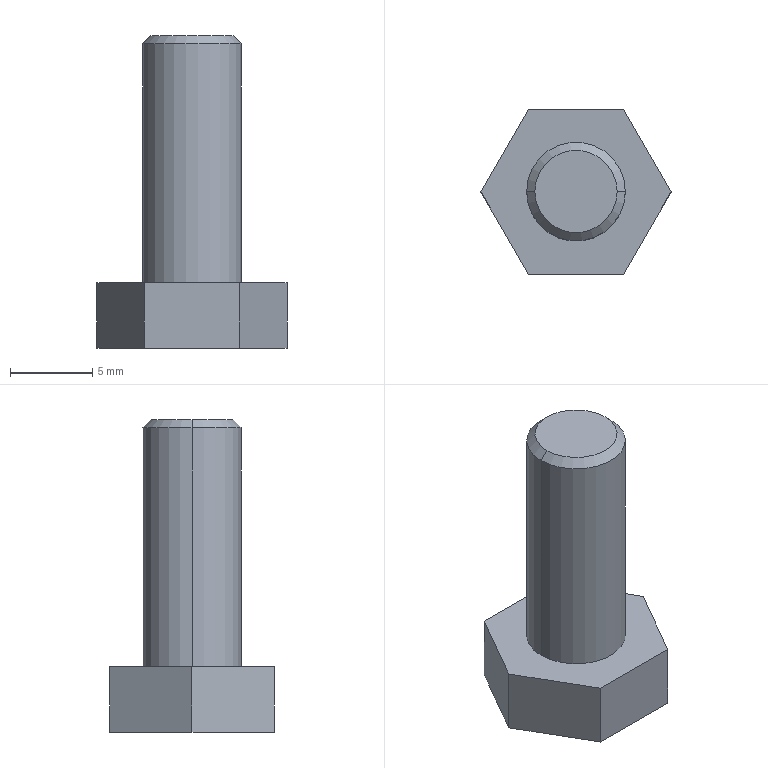Part | STEP file | Bulong M6_1.5F | 1 solid | 13 faces | box 11.547 x 10 x 19 mm | volume 768.3 mm3 | plane 9 | cone 2 | cylinder 2 | commonest cylinder face diameters 6 x2
STEP:
#1=CARTESIAN_POINT('',(0.,0.,0.));
#2=DIRECTION('',(0.,0.,1.));
#3=DIRECTION('',(1.,0.,0.));
#4=AXIS2_PLACEMENT_3D('',#1,#2,#3);
#5=CARTESIAN_POINT('',(2.5,0.,15.));
#6=VERTEX_POINT('',#5);
#7=CARTESIAN_POINT('',(-2.5,0.,15.));
#8=VERTEX_POINT('',#7);
#9=CARTESIAN_POINT('',(0.,0.,15.));
#10=DIRECTION('',(0.,0.,1.));
#11=DIRECTION('',(1.,0.,0.));
#12=AXIS2_PLACEMENT_3D('',#9,#10,#11);
#13=CIRCLE('',#12,2.5);
#14=CARTESIAN_POINT('',(0.,0.,15.));
#15=DIRECTION('',(0.,0.,-1.));
#16=DIRECTION('',(-1.,0.,0.));
#17=AXIS2_PLACEMENT_3D('',#14,#15,#16);
#18=CONICAL_SURFACE('',#17,2.5,0.7854);
#19=CARTESIAN_POINT('',(3.142,0.));
#20=DIRECTION('',(-1.,0.));
#21=VECTOR('',#20,1.);
#22=LINE('',#19,#21);
#23=(GEOMETRIC_REPRESENTATION_CONTEXT(2)PARAMETRIC_REPRESENTATION_CONTEXT()REPRESENTATION_CONTEXT('',''));
#24=DEFINITIONAL_REPRESENTATION('',(#22),#23);
#25=PCURVE('',#18,#24);
#26=CARTESIAN_POINT('',(0.,0.,15.));
#27=DIRECTION('',(0.,0.,1.));
#28=DIRECTION('',(1.,0.,0.));
#29=AXIS2_PLACEMENT_3D('',#26,#27,#28);
#30=PLANE('',#29);
#31=CARTESIAN_POINT('',(0.,0.));
#32=DIRECTION('',(1.,0.));
#33=AXIS2_PLACEMENT_2D('',#31,#32);
#34=CIRCLE('',#33,2.5);
#35=(GEOMETRIC_REPRESENTATION_CONTEXT(2)PARAMETRIC_REPRESENTATION_CONTEXT()REPRESENTATION_CONTEXT('',''));
#36=DEFINITIONAL_REPRESENTATION('',(#34),#35);
#37=PCURVE('',#30,#36);
#38=SURFACE_CURVE('',#13,(#25,#37),.PCURVE_S1.);
#39=EDGE_CURVE('',#6,#8,#38,.T.);
#40=ORIENTED_EDGE('',*,*,#39,.F.);
#41=CARTESIAN_POINT('',(3.,0.,14.5));
#42=VERTEX_POINT('',#41);
#43=CARTESIAN_POINT('',(2.5,0.,15.));
#44=DIRECTION('',(0.7071,0.,-0.7071));
#45=VECTOR('',#44,1.);
#46=LINE('',#43,#45);
#47=CARTESIAN_POINT('',(3.142,0.));
#48=DIRECTION('',(0.,1.));
#49=VECTOR('',#48,1.);
#50=LINE('',#47,#49);
#51=(GEOMETRIC_REPRESENTATION_CONTEXT(2)PARAMETRIC_REPRESENTATION_CONTEXT()REPRESENTATION_CONTEXT('',''));
#52=DEFINITIONAL_REPRESENTATION('',(#50),#51);
#53=PCURVE('',#18,#52);
#54=CARTESIAN_POINT('',(0.,0.,15.));
#55=DIRECTION('',(0.,0.,-1.));
#56=DIRECTION('',(-1.,0.,0.));
#57=AXIS2_PLACEMENT_3D('',#54,#55,#56);
#58=CONICAL_SURFACE('',#57,2.5,0.7854);
#59=CARTESIAN_POINT('',(3.142,0.));
#60=DIRECTION('',(0.,1.));
#61=VECTOR('',#60,1.);
#62=LINE('',#59,#61);
#63=(GEOMETRIC_REPRESENTATION_CONTEXT(2)PARAMETRIC_REPRESENTATION_CONTEXT()REPRESENTATION_CONTEXT('',''));
#64=DEFINITIONAL_REPRESENTATION('',(#62),#63);
#65=PCURVE('',#58,#64);
#66=SURFACE_CURVE('',#46,(#53,#65),.PCURVE_S1.);
#67=EDGE_CURVE('',#6,#42,#66,.T.);
#68=ORIENTED_EDGE('',*,*,#67,.T.);
#69=CARTESIAN_POINT('',(-3.,0.,14.5));
#70=VERTEX_POINT('',#69);
#71=CARTESIAN_POINT('',(0.,0.,14.5));
#72=DIRECTION('',(0.,0.,-1.));
#73=DIRECTION('',(1.,0.,0.));
#74=AXIS2_PLACEMENT_3D('',#71,#72,#73);
#75=CIRCLE('',#74,3.);
#76=CARTESIAN_POINT('',(-3.142,0.5));
#77=DIRECTION('',(1.,0.));
#78=VECTOR('',#77,1.);
#79=LINE('',#76,#78);
#80=(GEOMETRIC_REPRESENTATION_CONTEXT(2)PARAMETRIC_REPRESENTATION_CONTEXT()REPRESENTATION_CONTEXT('',''));
#81=DEFINITIONAL_REPRESENTATION('',(#79),#80);
#82=PCURVE('',#18,#81);
#83=CARTESIAN_POINT('',(0.,0.,15.));
#84=DIRECTION('',(0.,0.,-1.));
#85=DIRECTION('',(-1.,0.,0.));
#86=AXIS2_PLACEMENT_3D('',#83,#84,#85);
#87=CYLINDRICAL_SURFACE('',#86,3.);
#88=CARTESIAN_POINT('',(-3.142,0.5));
#89=DIRECTION('',(1.,0.));
#90=VECTOR('',#89,1.);
#91=LINE('',#88,#90);
#92=(GEOMETRIC_REPRESENTATION_CONTEXT(2)PARAMETRIC_REPRESENTATION_CONTEXT()REPRESENTATION_CONTEXT('',''));
#93=DEFINITIONAL_REPRESENTATION('',(#91),#92);
#94=PCURVE('',#87,#93);
#95=SURFACE_CURVE('',#75,(#82,#94),.PCURVE_S1.);
#96=EDGE_CURVE('',#70,#42,#95,.T.);
#97=ORIENTED_EDGE('',*,*,#96,.F.);
#98=CARTESIAN_POINT('',(-2.5,0.,15.));
#99=DIRECTION('',(-0.7071,0.,-0.7071));
#100=VECTOR('',#99,1.);
#101=LINE('',#98,#100);
#102=CARTESIAN_POINT('',(0.,0.));
#103=DIRECTION('',(0.,1.));
#104=VECTOR('',#103,1.);
#105=LINE('',#102,#104);
#106=(GEOMETRIC_REPRESENTATION_CONTEXT(2)PARAMETRIC_REPRESENTATION_CONTEXT()REPRESENTATION_CONTEXT('',''));
#107=DEFINITIONAL_REPRESENTATION('',(#105),#106);
#108=PCURVE('',#18,#107);
#109=CARTESIAN_POINT('',(6.283,0.));
#110=DIRECTION('',(0.,1.));
#111=VECTOR('',#110,1.);
#112=LINE('',#109,#111);
#113=(GEOMETRIC_REPRESENTATION_CONTEXT(2)PARAMETRIC_REPRESENTATION_CONTEXT()REPRESENTATION_CONTEXT('',''));
#114=DEFINITIONAL_REPRESENTATION('',(#112),#113);
#115=PCURVE('',#58,#114);
#116=SURFACE_CURVE('',#101,(#108,#115),.PCURVE_S1.);
#117=EDGE_CURVE('',#8,#70,#116,.T.);
#118=ORIENTED_EDGE('',*,*,#117,.F.);
#119=EDGE_LOOP('',(#40,#68,#97,#118));
#120=FACE_BOUND('',#119,.T.);
#121=ADVANCED_FACE('',(#120),#18,.T.);
#122=ORIENTED_EDGE('',*,*,#96,.T.);
#123=CARTESIAN_POINT('',(3.,0.,0.));
#124=VERTEX_POINT('',#123);
#125=CARTESIAN_POINT('',(3.,0.,15.));
#126=DIRECTION('',(0.,0.,-1.));
#127=VECTOR('',#126,1.);
#128=LINE('',#125,#127);
#129=CARTESIAN_POINT('',(3.142,0.));
#130=DIRECTION('',(0.,1.));
#131=VECTOR('',#130,1.);
#132=LINE('',#129,#131);
#133=(GEOMETRIC_REPRESENTATION_CONTEXT(2)PARAMETRIC_REPRESENTATION_CONTEXT()REPRESENTATION_CONTEXT('',''));
#134=DEFINITIONAL_REPRESENTATION('',(#132),#133);
#135=PCURVE('',#87,#134);
#136=CARTESIAN_POINT('',(0.,0.,15.));
#137=DIRECTION('',(0.,0.,-1.));
#138=DIRECTION('',(-1.,0.,0.));
#139=AXIS2_PLACEMENT_3D('',#136,#137,#138);
#140=CYLINDRICAL_SURFACE('',#139,3.);
#141=CARTESIAN_POINT('',(3.142,0.));
#142=DIRECTION('',(0.,1.));
#143=VECTOR('',#142,1.);
#144=LINE('',#141,#143);
#145=(GEOMETRIC_REPRESENTATION_CONTEXT(2)PARAMETRIC_REPRESENTATION_CONTEXT()REPRESENTATION_CONTEXT('',''));
#146=DEFINITIONAL_REPRESENTATION('',(#144),#145);
#147=PCURVE('',#140,#146);
#148=SURFACE_CURVE('',#128,(#135,#147),.PCURVE_S1.);
#149=EDGE_CURVE('',#42,#124,#148,.T.);
#150=ORIENTED_EDGE('',*,*,#149,.T.);
#151=CARTESIAN_POINT('',(-3.,0.,0.));
#152=VERTEX_POINT('',#151);
#153=CARTESIAN_POINT('',(0.,0.,0.));
#154=DIRECTION('',(0.,0.,1.));
#155=DIRECTION('',(1.,0.,0.));
#156=AXIS2_PLACEMENT_3D('',#153,#154,#155);
#157=CIRCLE('',#156,3.);
#158=CARTESIAN_POINT('',(3.142,15.));
#159=DIRECTION('',(-1.,0.));
#160=VECTOR('',#159,1.);
#161=LINE('',#158,#160);
#162=(GEOMETRIC_REPRESENTATION_CONTEXT(2)PARAMETRIC_REPRESENTATION_CONTEXT()REPRESENTATION_CONTEXT('',''));
#163=DEFINITIONAL_REPRESENTATION('',(#161),#162);
#164=PCURVE('',#87,#163);
#165=CARTESIAN_POINT('',(0.,0.,0.));
#166=DIRECTION('',(0.,0.,1.));
#167=DIRECTION('',(1.,0.,0.));
#168=AXIS2_PLACEMENT_3D('',#165,#166,#167);
#169=PLANE('',#168);
#170=CARTESIAN_POINT('',(0.,0.));
#171=DIRECTION('',(1.,0.));
#172=AXIS2_PLACEMENT_2D('',#170,#171);
#173=CIRCLE('',#172,3.);
#174=(GEOMETRIC_REPRESENTATION_CONTEXT(2)PARAMETRIC_REPRESENTATION_CONTEXT()REPRESENTATION_CONTEXT('',''));
#175=DEFINITIONAL_REPRESENTATION('',(#173),#174);
#176=PCURVE('',#169,#175);
#177=SURFACE_CURVE('',#157,(#164,#176),.PCURVE_S1.);
#178=EDGE_CURVE('',#124,#152,#177,.T.);
#179=ORIENTED_EDGE('',*,*,#178,.T.);
#180=CARTESIAN_POINT('',(-3.,0.,15.));
#181=DIRECTION('',(0.,0.,-1.));
#182=VECTOR('',#181,1.);
#183=LINE('',#180,#182);
#184=CARTESIAN_POINT('',(0.,0.));
#185=DIRECTION('',(0.,1.));
#186=VECTOR('',#185,1.);
#187=LINE('',#184,#186);
#188=(GEOMETRIC_REPRESENTATION_CONTEXT(2)PARAMETRIC_REPRESENTATION_CONTEXT()REPRESENTATION_CONTEXT('',''));
#189=DEFINITIONAL_REPRESENTATION('',(#187),#188);
#190=PCURVE('',#87,#189);
#191=CARTESIAN_POINT('',(6.283,0.));
#192=DIRECTION('',(0.,1.));
#193=VECTOR('',#192,1.);
#194=LINE('',#191,#193);
#195=(GEOMETRIC_REPRESENTATION_CONTEXT(2)PARAMETRIC_REPRESENTATION_CONTEXT()REPRESENTATION_CONTEXT('',''));
#196=DEFINITIONAL_REPRESENTATION('',(#194),#195);
#197=PCURVE('',#140,#196);
#198=SURFACE_CURVE('',#183,(#190,#197),.PCURVE_S1.);
#199=EDGE_CURVE('',#70,#152,#198,.T.);
#200=ORIENTED_EDGE('',*,*,#199,.F.);
#201=EDGE_LOOP('',(#122,#150,#179,#200));
#202=FACE_BOUND('',#201,.T.);
#203=ADVANCED_FACE('',(#202),#87,.T.);
#204=CARTESIAN_POINT('',(-2.887,5.,0.));
#205=VERTEX_POINT('',#204);
#206=CARTESIAN_POINT('',(-5.774,0.,0.));
#207=VERTEX_POINT('',#206);
#208=CARTESIAN_POINT('',(-2.887,5.,0.));
#209=DIRECTION('',(-0.5,-0.866,0.));
#210=VECTOR('',#209,1.);
#211=LINE('',#208,#210);
#212=CARTESIAN_POINT('',(-2.887,5.));
#213=DIRECTION('',(-0.5,-0.866));
#214=VECTOR('',#213,1.);
#215=LINE('',#212,#214);
#216=(GEOMETRIC_REPRESENTATION_CONTEXT(2)PARAMETRIC_REPRESENTATION_CONTEXT()REPRESENTATION_CONTEXT('',''));
#217=DEFINITIONAL_REPRESENTATION('',(#215),#216);
#218=PCURVE('',#169,#217);
#219=CARTESIAN_POINT('',(-2.887,5.,-4.));
#220=DIRECTION('',(-0.866,0.5,0.));
#221=DIRECTION('',(-0.5,-0.866,0.));
#222=AXIS2_PLACEMENT_3D('',#219,#220,#221);
#223=PLANE('',#222);
#224=CARTESIAN_POINT('',(0.,4.));
#225=DIRECTION('',(1.,0.));
#226=VECTOR('',#225,1.);
#227=LINE('',#224,#226);
#228=(GEOMETRIC_REPRESENTATION_CONTEXT(2)PARAMETRIC_REPRESENTATION_CONTEXT()REPRESENTATION_CONTEXT('',''));
#229=DEFINITIONAL_REPRESENTATION('',(#227),#228);
#230=PCURVE('',#223,#229);
#231=SURFACE_CURVE('',#211,(#218,#230),.PCURVE_S1.);
#232=EDGE_CURVE('',#205,#207,#231,.T.);
#233=ORIENTED_EDGE('',*,*,#232,.T.);
#234=CARTESIAN_POINT('',(-2.887,-5.,0.));
#235=VERTEX_POINT('',#234);
#236=CARTESIAN_POINT('',(-5.774,0.,0.));
#237=DIRECTION('',(0.5,-0.866,0.));
#238=VECTOR('',#237,1.);
#239=LINE('',#236,#238);
#240=CARTESIAN_POINT('',(-5.774,0.));
#241=DIRECTION('',(0.5,-0.866));
#242=VECTOR('',#241,1.);
#243=LINE('',#240,#242);
#244=(GEOMETRIC_REPRESENTATION_CONTEXT(2)PARAMETRIC_REPRESENTATION_CONTEXT()REPRESENTATION_CONTEXT('',''));
#245=DEFINITIONAL_REPRESENTATION('',(#243),#244);
#246=PCURVE('',#169,#245);
#247=CARTESIAN_POINT('',(-5.774,0.,-4.));
#248=DIRECTION('',(-0.866,-0.5,0.));
#249=DIRECTION('',(0.5,-0.866,0.));
#250=AXIS2_PLACEMENT_3D('',#247,#248,#249);
#251=PLANE('',#250);
#252=CARTESIAN_POINT('',(0.,4.));
#253=DIRECTION('',(1.,0.));
#254=VECTOR('',#253,1.);
#255=LINE('',#252,#254);
#256=(GEOMETRIC_REPRESENTATION_CONTEXT(2)PARAMETRIC_REPRESENTATION_CONTEXT()REPRESENTATION_CONTEXT('',''));
#257=DEFINITIONAL_REPRESENTATION('',(#255),#256);
#258=PCURVE('',#251,#257);
#259=SURFACE_CURVE('',#239,(#246,#258),.PCURVE_S1.);
#260=EDGE_CURVE('',#207,#235,#259,.T.);
#261=ORIENTED_EDGE('',*,*,#260,.T.);
#262=CARTESIAN_POINT('',(2.887,-5.,0.));
#263=VERTEX_POINT('',#262);
#264=CARTESIAN_POINT('',(-2.887,-5.,0.));
#265=DIRECTION('',(1.,0.,0.));
#266=VECTOR('',#265,1.);
#267=LINE('',#264,#266);
#268=CARTESIAN_POINT('',(-2.887,-5.));
#269=DIRECTION('',(1.,0.));
#270=VECTOR('',#269,1.);
#271=LINE('',#268,#270);
#272=(GEOMETRIC_REPRESENTATION_CONTEXT(2)PARAMETRIC_REPRESENTATION_CONTEXT()REPRESENTATION_CONTEXT('',''));
#273=DEFINITIONAL_REPRESENTATION('',(#271),#272);
#274=PCURVE('',#169,#273);
#275=CARTESIAN_POINT('',(-2.887,-5.,-4.));
#276=DIRECTION('',(0.,-1.,0.));
#277=DIRECTION('',(1.,0.,0.));
#278=AXIS2_PLACEMENT_3D('',#275,#276,#277);
#279=PLANE('',#278);
#280=CARTESIAN_POINT('',(0.,4.));
#281=DIRECTION('',(1.,0.));
#282=VECTOR('',#281,1.);
#283=LINE('',#280,#282);
#284=(GEOMETRIC_REPRESENTATION_CONTEXT(2)PARAMETRIC_REPRESENTATION_CONTEXT()REPRESENTATION_CONTEXT('',''));
#285=DEFINITIONAL_REPRESENTATION('',(#283),#284);
#286=PCURVE('',#279,#285);
#287=SURFACE_CURVE('',#267,(#274,#286),.PCURVE_S1.);
#288=EDGE_CURVE('',#235,#263,#287,.T.);
#289=ORIENTED_EDGE('',*,*,#288,.T.);
#290=CARTESIAN_POINT('',(5.774,0.,0.));
#291=VERTEX_POINT('',#290);
#292=CARTESIAN_POINT('',(2.887,-5.,0.));
#293=DIRECTION('',(0.5,0.866,0.));
#294=VECTOR('',#293,1.);
#295=LINE('',#292,#294);
#296=CARTESIAN_POINT('',(2.887,-5.));
#297=DIRECTION('',(0.5,0.866));
#298=VECTOR('',#297,1.);
#299=LINE('',#296,#298);
#300=(GEOMETRIC_REPRESENTATION_CONTEXT(2)PARAMETRIC_REPRESENTATION_CONTEXT()REPRESENTATION_CONTEXT('',''));
#301=DEFINITIONAL_REPRESENTATION('',(#299),#300);
#302=PCURVE('',#169,#301);
#303=CARTESIAN_POINT('',(2.887,-5.,-4.));
#304=DIRECTION('',(0.866,-0.5,0.));
#305=DIRECTION('',(0.5,0.866,0.));
#306=AXIS2_PLACEMENT_3D('',#303,#304,#305);
#307=PLANE('',#306);
#308=CARTESIAN_POINT('',(0.,4.));
#309=DIRECTION('',(1.,0.));
#310=VECTOR('',#309,1.);
#311=LINE('',#308,#310);
#312=(GEOMETRIC_REPRESENTATION_CONTEXT(2)PARAMETRIC_REPRESENTATION_CONTEXT()REPRESENTATION_CONTEXT('',''));
#313=DEFINITIONAL_REPRESENTATION('',(#311),#312);
#314=PCURVE('',#307,#313);
#315=SURFACE_CURVE('',#295,(#302,#314),.PCURVE_S1.);
#316=EDGE_CURVE('',#263,#291,#315,.T.);
#317=ORIENTED_EDGE('',*,*,#316,.T.);
#318=CARTESIAN_POINT('',(2.887,5.,0.));
#319=VERTEX_POINT('',#318);
#320=CARTESIAN_POINT('',(5.774,0.,0.));
#321=DIRECTION('',(-0.5,0.866,0.));
#322=VECTOR('',#321,1.);
#323=LINE('',#320,#322);
#324=CARTESIAN_POINT('',(5.774,0.));
#325=DIRECTION('',(-0.5,0.866));
#326=VECTOR('',#325,1.);
#327=LINE('',#324,#326);
#328=(GEOMETRIC_REPRESENTATION_CONTEXT(2)PARAMETRIC_REPRESENTATION_CONTEXT()REPRESENTATION_CONTEXT('',''));
#329=DEFINITIONAL_REPRESENTATION('',(#327),#328);
#330=PCURVE('',#169,#329);
#331=CARTESIAN_POINT('',(5.774,0.,-4.));
#332=DIRECTION('',(0.866,0.5,0.));
#333=DIRECTION('',(-0.5,0.866,0.));
#334=AXIS2_PLACEMENT_3D('',#331,#332,#333);
#335=PLANE('',#334);
#336=CARTESIAN_POINT('',(0.,4.));
#337=DIRECTION('',(1.,0.));
#338=VECTOR('',#337,1.);
#339=LINE('',#336,#338);
#340=(GEOMETRIC_REPRESENTATION_CONTEXT(2)PARAMETRIC_REPRESENTATION_CONTEXT()REPRESENTATION_CONTEXT('',''));
#341=DEFINITIONAL_REPRESENTATION('',(#339),#340);
#342=PCURVE('',#335,#341);
#343=SURFACE_CURVE('',#323,(#330,#342),.PCURVE_S1.);
#344=EDGE_CURVE('',#291,#319,#343,.T.);
#345=ORIENTED_EDGE('',*,*,#344,.T.);
#346=CARTESIAN_POINT('',(2.887,5.,0.));
#347=DIRECTION('',(-1.,0.,0.));
#348=VECTOR('',#347,1.);
#349=LINE('',#346,#348);
#350=CARTESIAN_POINT('',(2.887,5.));
#351=DIRECTION('',(-1.,0.));
#352=VECTOR('',#351,1.);
#353=LINE('',#350,#352);
#354=(GEOMETRIC_REPRESENTATION_CONTEXT(2)PARAMETRIC_REPRESENTATION_CONTEXT()REPRESENTATION_CONTEXT('',''));
#355=DEFINITIONAL_REPRESENTATION('',(#353),#354);
#356=PCURVE('',#169,#355);
#357=CARTESIAN_POINT('',(2.887,5.,-4.));
#358=DIRECTION('',(0.,1.,0.));
#359=DIRECTION('',(0.,0.,1.));
#360=AXIS2_PLACEMENT_3D('',#357,#358,#359);
#361=PLANE('',#360);
#362=CARTESIAN_POINT('',(4.,0.));
#363=DIRECTION('',(0.,-1.));
#364=VECTOR('',#363,1.);
#365=LINE('',#362,#364);
#366=(GEOMETRIC_REPRESENTATION_CONTEXT(2)PARAMETRIC_REPRESENTATION_CONTEXT()REPRESENTATION_CONTEXT('',''));
#367=DEFINITIONAL_REPRESENTATION('',(#365),#366);
#368=PCURVE('',#361,#367);
#369=SURFACE_CURVE('',#349,(#356,#368),.PCURVE_S1.);
#370=EDGE_CURVE('',#319,#205,#369,.T.);
#371=ORIENTED_EDGE('',*,*,#370,.T.);
#372=EDGE_LOOP('',(#233,#261,#289,#317,#345,#371));
#373=FACE_BOUND('',#372,.T.);
#374=CARTESIAN_POINT('',(0.,0.,0.));
#375=DIRECTION('',(0.,0.,1.));
#376=DIRECTION('',(1.,0.,0.));
#377=AXIS2_PLACEMENT_3D('',#374,#375,#376);
#378=CIRCLE('',#377,3.);
#379=CARTESIAN_POINT('',(0.,0.));
#380=DIRECTION('',(1.,0.));
#381=AXIS2_PLACEMENT_2D('',#379,#380);
#382=CIRCLE('',#381,3.);
#383=(GEOMETRIC_REPRESENTATION_CONTEXT(2)PARAMETRIC_REPRESENTATION_CONTEXT()REPRESENTATION_CONTEXT('',''));
#384=DEFINITIONAL_REPRESENTATION('',(#382),#383);
#385=PCURVE('',#169,#384);
#386=CARTESIAN_POINT('',(9.425,15.));
#387=DIRECTION('',(-1.,0.));
#388=VECTOR('',#387,1.);
#389=LINE('',#386,#388);
#390=(GEOMETRIC_REPRESENTATION_CONTEXT(2)PARAMETRIC_REPRESENTATION_CONTEXT()REPRESENTATION_CONTEXT('',''));
#391=DEFINITIONAL_REPRESENTATION('',(#389),#390);
#392=PCURVE('',#140,#391);
#393=SURFACE_CURVE('',#378,(#385,#392),.PCURVE_S1.);
#394=EDGE_CURVE('',#152,#124,#393,.T.);
#395=ORIENTED_EDGE('',*,*,#394,.F.);
#396=ORIENTED_EDGE('',*,*,#178,.F.);
#397=EDGE_LOOP('',(#395,#396));
#398=FACE_BOUND('',#397,.T.);
#399=ADVANCED_FACE('',(#373,#398),#169,.T.);
#400=ORIENTED_EDGE('',*,*,#232,.F.);
#401=CARTESIAN_POINT('',(-2.887,5.,-4.));
#402=VERTEX_POINT('',#401);
#403=CARTESIAN_POINT('',(-2.887,5.,-4.));
#404=DIRECTION('',(0.,0.,1.));
#405=VECTOR('',#404,1.);
#406=LINE('',#403,#405);
#407=CARTESIAN_POINT('',(0.,0.));
#408=DIRECTION('',(0.,1.));
#409=VECTOR('',#408,1.);
#410=LINE('',#407,#409);
#411=(GEOMETRIC_REPRESENTATION_CONTEXT(2)PARAMETRIC_REPRESENTATION_CONTEXT()REPRESENTATION_CONTEXT('',''));
#412=DEFINITIONAL_REPRESENTATION('',(#410),#411);
#413=PCURVE('',#223,#412);
#414=CARTESIAN_POINT('',(0.,-5.774));
#415=DIRECTION('',(1.,0.));
#416=VECTOR('',#415,1.);
#417=LINE('',#414,#416);
#418=(GEOMETRIC_REPRESENTATION_CONTEXT(2)PARAMETRIC_REPRESENTATION_CONTEXT()REPRESENTATION_CONTEXT('',''));
#419=DEFINITIONAL_REPRESENTATION('',(#417),#418);
#420=PCURVE('',#361,#419);
#421=SURFACE_CURVE('',#406,(#413,#420),.PCURVE_S1.);
#422=EDGE_CURVE('',#402,#205,#421,.T.);
#423=ORIENTED_EDGE('',*,*,#422,.F.);
#424=CARTESIAN_POINT('',(-5.774,0.,-4.));
#425=VERTEX_POINT('',#424);
#426=CARTESIAN_POINT('',(-2.887,5.,-4.));
#427=DIRECTION('',(-0.5,-0.866,0.));
#428=VECTOR('',#427,1.);
#429=LINE('',#426,#428);
#430=CARTESIAN_POINT('',(0.,0.));
#431=DIRECTION('',(1.,0.));
#432=VECTOR('',#431,1.);
#433=LINE('',#430,#432);
#434=(GEOMETRIC_REPRESENTATION_CONTEXT(2)PARAMETRIC_REPRESENTATION_CONTEXT()REPRESENTATION_CONTEXT('',''));
#435=DEFINITIONAL_REPRESENTATION('',(#433),#434);
#436=PCURVE('',#223,#435);
#437=CARTESIAN_POINT('',(0.,0.,-4.));
#438=DIRECTION('',(0.,0.,1.));
#439=DIRECTION('',(1.,0.,0.));
#440=AXIS2_PLACEMENT_3D('',#437,#438,#439);
#441=PLANE('',#440);
#442=CARTESIAN_POINT('',(-2.887,5.));
#443=DIRECTION('',(-0.5,-0.866));
#444=VECTOR('',#443,1.);
#445=LINE('',#442,#444);
#446=(GEOMETRIC_REPRESENTATION_CONTEXT(2)PARAMETRIC_REPRESENTATION_CONTEXT()REPRESENTATION_CONTEXT('',''));
#447=DEFINITIONAL_REPRESENTATION('',(#445),#446);
#448=PCURVE('',#441,#447);
#449=SURFACE_CURVE('',#429,(#436,#448),.PCURVE_S1.);
#450=EDGE_CURVE('',#402,#425,#449,.T.);
#451=ORIENTED_EDGE('',*,*,#450,.T.);
#452=CARTESIAN_POINT('',(-5.774,0.,-4.));
#453=DIRECTION('',(0.,0.,1.));
#454=VECTOR('',#453,1.);
#455=LINE('',#452,#454);
#456=CARTESIAN_POINT('',(5.774,0.));
#457=DIRECTION('',(0.,1.));
#458=VECTOR('',#457,1.);
#459=LINE('',#456,#458);
#460=(GEOMETRIC_REPRESENTATION_CONTEXT(2)PARAMETRIC_REPRESENTATION_CONTEXT()REPRESENTATION_CONTEXT('',''));
#461=DEFINITIONAL_REPRESENTATION('',(#459),#460);
#462=PCURVE('',#223,#461);
#463=CARTESIAN_POINT('',(0.,0.));
#464=DIRECTION('',(0.,1.));
#465=VECTOR('',#464,1.);
#466=LINE('',#463,#465);
#467=(GEOMETRIC_REPRESENTATION_CONTEXT(2)PARAMETRIC_REPRESENTATION_CONTEXT()REPRESENTATION_CONTEXT('',''));
#468=DEFINITIONAL_REPRESENTATION('',(#466),#467);
#469=PCURVE('',#251,#468);
#470=SURFACE_CURVE('',#455,(#462,#469),.PCURVE_S1.);
#471=EDGE_CURVE('',#425,#207,#470,.T.);
#472=ORIENTED_EDGE('',*,*,#471,.T.);
#473=EDGE_LOOP('',(#400,#423,#451,#472));
#474=FACE_BOUND('',#473,.T.);
#475=ADVANCED_FACE('',(#474),#223,.T.);
#476=ORIENTED_EDGE('',*,*,#370,.F.);
#477=CARTESIAN_POINT('',(2.887,5.,-4.));
#478=VERTEX_POINT('',#477);
#479=CARTESIAN_POINT('',(2.887,5.,-4.));
#480=DIRECTION('',(0.,0.,1.));
#481=VECTOR('',#480,1.);
#482=LINE('',#479,#481);
#483=CARTESIAN_POINT('',(0.,0.));
#484=DIRECTION('',(1.,0.));
#485=VECTOR('',#484,1.);
#486=LINE('',#483,#485);
#487=(GEOMETRIC_REPRESENTATION_CONTEXT(2)PARAMETRIC_REPRESENTATION_CONTEXT()REPRESENTATION_CONTEXT('',''));
#488=DEFINITIONAL_REPRESENTATION('',(#486),#487);
#489=PCURVE('',#361,#488);
#490=CARTESIAN_POINT('',(5.774,0.));
#491=DIRECTION('',(0.,1.));
#492=VECTOR('',#491,1.);
#493=LINE('',#490,#492);
#494=(GEOMETRIC_REPRESENTATION_CONTEXT(2)PARAMETRIC_REPRESENTATION_CONTEXT()REPRESENTATION_CONTEXT('',''));
#495=DEFINITIONAL_REPRESENTATION('',(#493),#494);
#496=PCURVE('',#335,#495);
#497=SURFACE_CURVE('',#482,(#489,#496),.PCURVE_S1.);
#498=EDGE_CURVE('',#478,#319,#497,.T.);
#499=ORIENTED_EDGE('',*,*,#498,.F.);
#500=CARTESIAN_POINT('',(2.887,5.,-4.));
#501=DIRECTION('',(-1.,0.,0.));
#502=VECTOR('',#501,1.);
#503=LINE('',#500,#502);
#504=CARTESIAN_POINT('',(0.,0.));
#505=DIRECTION('',(0.,-1.));
#506=VECTOR('',#505,1.);
#507=LINE('',#504,#506);
#508=(GEOMETRIC_REPRESENTATION_CONTEXT(2)PARAMETRIC_REPRESENTATION_CONTEXT()REPRESENTATION_CONTEXT('',''));
#509=DEFINITIONAL_REPRESENTATION('',(#507),#508);
#510=PCURVE('',#361,#509);
#511=CARTESIAN_POINT('',(2.887,5.));
#512=DIRECTION('',(-1.,0.));
#513=VECTOR('',#512,1.);
#514=LINE('',#511,#513);
#515=(GEOMETRIC_REPRESENTATION_CONTEXT(2)PARAMETRIC_REPRESENTATION_CONTEXT()REPRESENTATION_CONTEXT('',''));
#516=DEFINITIONAL_REPRESENTATION('',(#514),#515);
#517=PCURVE('',#441,#516);
#518=SURFACE_CURVE('',#503,(#510,#517),.PCURVE_S1.);
#519=EDGE_CURVE('',#478,#402,#518,.T.);
#520=ORIENTED_EDGE('',*,*,#519,.T.);
#521=ORIENTED_EDGE('',*,*,#422,.T.);
#522=EDGE_LOOP('',(#476,#499,#520,#521));
#523=FACE_BOUND('',#522,.T.);
#524=ADVANCED_FACE('',(#523),#361,.T.);
#525=ORIENTED_EDGE('',*,*,#344,.F.);
#526=CARTESIAN_POINT('',(5.774,0.,-4.));
#527=VERTEX_POINT('',#526);
#528=CARTESIAN_POINT('',(5.774,0.,-4.));
#529=DIRECTION('',(0.,0.,1.));
#530=VECTOR('',#529,1.);
#531=LINE('',#528,#530);
#532=CARTESIAN_POINT('',(0.,0.));
#533=DIRECTION('',(0.,1.));
#534=VECTOR('',#533,1.);
#535=LINE('',#532,#534);
#536=(GEOMETRIC_REPRESENTATION_CONTEXT(2)PARAMETRIC_REPRESENTATION_CONTEXT()REPRESENTATION_CONTEXT('',''));
#537=DEFINITIONAL_REPRESENTATION('',(#535),#536);
#538=PCURVE('',#335,#537);
#539=CARTESIAN_POINT('',(5.774,0.));
#540=DIRECTION('',(0.,1.));
#541=VECTOR('',#540,1.);
#542=LINE('',#539,#541);
#543=(GEOMETRIC_REPRESENTATION_CONTEXT(2)PARAMETRIC_REPRESENTATION_CONTEXT()REPRESENTATION_CONTEXT('',''));
#544=DEFINITIONAL_REPRESENTATION('',(#542),#543);
#545=PCURVE('',#307,#544);
#546=SURFACE_CURVE('',#531,(#538,#545),.PCURVE_S1.);
#547=EDGE_CURVE('',#527,#291,#546,.T.);
#548=ORIENTED_EDGE('',*,*,#547,.F.);
#549=CARTESIAN_POINT('',(5.774,0.,-4.));
#550=DIRECTION('',(-0.5,0.866,0.));
#551=VECTOR('',#550,1.);
#552=LINE('',#549,#551);
#553=CARTESIAN_POINT('',(0.,0.));
#554=DIRECTION('',(1.,0.));
#555=VECTOR('',#554,1.);
#556=LINE('',#553,#555);
#557=(GEOMETRIC_REPRESENTATION_CONTEXT(2)PARAMETRIC_REPRESENTATION_CONTEXT()REPRESENTATION_CONTEXT('',''));
#558=DEFINITIONAL_REPRESENTATION('',(#556),#557);
#559=PCURVE('',#335,#558);
#560=CARTESIAN_POINT('',(5.774,0.));
#561=DIRECTION('',(-0.5,0.866));
#562=VECTOR('',#561,1.);
#563=LINE('',#560,#562);
#564=(GEOMETRIC_REPRESENTATION_CONTEXT(2)PARAMETRIC_REPRESENTATION_CONTEXT()REPRESENTATION_CONTEXT('',''));
#565=DEFINITIONAL_REPRESENTATION('',(#563),#564);
#566=PCURVE('',#441,#565);
#567=SURFACE_CURVE('',#552,(#559,#566),.PCURVE_S1.);
#568=EDGE_CURVE('',#527,#478,#567,.T.);
#569=ORIENTED_EDGE('',*,*,#568,.T.);
#570=ORIENTED_EDGE('',*,*,#498,.T.);
#571=EDGE_LOOP('',(#525,#548,#569,#570));
#572=FACE_BOUND('',#571,.T.);
#573=ADVANCED_FACE('',(#572),#335,.T.);
#574=ORIENTED_EDGE('',*,*,#316,.F.);
#575=CARTESIAN_POINT('',(2.887,-5.,-4.));
#576=VERTEX_POINT('',#575);
#577=CARTESIAN_POINT('',(2.887,-5.,-4.));
#578=DIRECTION('',(0.,0.,1.));
#579=VECTOR('',#578,1.);
#580=LINE('',#577,#579);
#581=CARTESIAN_POINT('',(0.,0.));
#582=DIRECTION('',(0.,1.));
#583=VECTOR('',#582,1.);
#584=LINE('',#581,#583);
#585=(GEOMETRIC_REPRESENTATION_CONTEXT(2)PARAMETRIC_REPRESENTATION_CONTEXT()REPRESENTATION_CONTEXT('',''));
#586=DEFINITIONAL_REPRESENTATION('',(#584),#585);
#587=PCURVE('',#307,#586);
#588=CARTESIAN_POINT('',(5.774,0.));
#589=DIRECTION('',(0.,1.));
#590=VECTOR('',#589,1.);
#591=LINE('',#588,#590);
#592=(GEOMETRIC_REPRESENTATION_CONTEXT(2)PARAMETRIC_REPRESENTATION_CONTEXT()REPRESENTATION_CONTEXT('',''));
#593=DEFINITIONAL_REPRESENTATION('',(#591),#592);
#594=PCURVE('',#279,#593);
#595=SURFACE_CURVE('',#580,(#587,#594),.PCURVE_S1.);
#596=EDGE_CURVE('',#576,#263,#595,.T.);
#597=ORIENTED_EDGE('',*,*,#596,.F.);
#598=CARTESIAN_POINT('',(2.887,-5.,-4.));
#599=DIRECTION('',(0.5,0.866,0.));
#600=VECTOR('',#599,1.);
#601=LINE('',#598,#600);
#602=CARTESIAN_POINT('',(0.,0.));
#603=DIRECTION('',(1.,0.));
#604=VECTOR('',#603,1.);
#605=LINE('',#602,#604);
#606=(GEOMETRIC_REPRESENTATION_CONTEXT(2)PARAMETRIC_REPRESENTATION_CONTEXT()REPRESENTATION_CONTEXT('',''));
#607=DEFINITIONAL_REPRESENTATION('',(#605),#606);
#608=PCURVE('',#307,#607);
#609=CARTESIAN_POINT('',(2.887,-5.));
#610=DIRECTION('',(0.5,0.866));
#611=VECTOR('',#610,1.);
#612=LINE('',#609,#611);
#613=(GEOMETRIC_REPRESENTATION_CONTEXT(2)PARAMETRIC_REPRESENTATION_CONTEXT()REPRESENTATION_CONTEXT('',''));
#614=DEFINITIONAL_REPRESENTATION('',(#612),#613);
#615=PCURVE('',#441,#614);
#616=SURFACE_CURVE('',#601,(#608,#615),.PCURVE_S1.);
#617=EDGE_CURVE('',#576,#527,#616,.T.);
#618=ORIENTED_EDGE('',*,*,#617,.T.);
#619=ORIENTED_EDGE('',*,*,#547,.T.);
#620=EDGE_LOOP('',(#574,#597,#618,#619));
#621=FACE_BOUND('',#620,.T.);
#622=ADVANCED_FACE('',(#621),#307,.T.);
#623=ORIENTED_EDGE('',*,*,#288,.F.);
#624=CARTESIAN_POINT('',(-2.887,-5.,-4.));
#625=VERTEX_POINT('',#624);
#626=CARTESIAN_POINT('',(-2.887,-5.,-4.));
#627=DIRECTION('',(0.,0.,1.));
#628=VECTOR('',#627,1.);
#629=LINE('',#626,#628);
#630=CARTESIAN_POINT('',(0.,0.));
#631=DIRECTION('',(0.,1.));
#632=VECTOR('',#631,1.);
#633=LINE('',#630,#632);
#634=(GEOMETRIC_REPRESENTATION_CONTEXT(2)PARAMETRIC_REPRESENTATION_CONTEXT()REPRESENTATION_CONTEXT('',''));
#635=DEFINITIONAL_REPRESENTATION('',(#633),#634);
#636=PCURVE('',#279,#635);
#637=CARTESIAN_POINT('',(5.774,0.));
#638=DIRECTION('',(0.,1.));
#639=VECTOR('',#638,1.);
#640=LINE('',#637,#639);
#641=(GEOMETRIC_REPRESENTATION_CONTEXT(2)PARAMETRIC_REPRESENTATION_CONTEXT()REPRESENTATION_CONTEXT('',''));
#642=DEFINITIONAL_REPRESENTATION('',(#640),#641);
#643=PCURVE('',#251,#642);
#644=SURFACE_CURVE('',#629,(#636,#643),.PCURVE_S1.);
#645=EDGE_CURVE('',#625,#235,#644,.T.);
#646=ORIENTED_EDGE('',*,*,#645,.F.);
#647=CARTESIAN_POINT('',(-2.887,-5.,-4.));
#648=DIRECTION('',(1.,0.,0.));
#649=VECTOR('',#648,1.);
#650=LINE('',#647,#649);
#651=CARTESIAN_POINT('',(0.,0.));
#652=DIRECTION('',(1.,0.));
#653=VECTOR('',#652,1.);
#654=LINE('',#651,#653);
#655=(GEOMETRIC_REPRESENTATION_CONTEXT(2)PARAMETRIC_REPRESENTATION_CONTEXT()REPRESENTATION_CONTEXT('',''));
#656=DEFINITIONAL_REPRESENTATION('',(#654),#655);
#657=PCURVE('',#279,#656);
#658=CARTESIAN_POINT('',(-2.887,-5.));
#659=DIRECTION('',(1.,0.));
#660=VECTOR('',#659,1.);
#661=LINE('',#658,#660);
#662=(GEOMETRIC_REPRESENTATION_CONTEXT(2)PARAMETRIC_REPRESENTATION_CONTEXT()REPRESENTATION_CONTEXT('',''));
#663=DEFINITIONAL_REPRESENTATION('',(#661),#662);
#664=PCURVE('',#441,#663);
#665=SURFACE_CURVE('',#650,(#657,#664),.PCURVE_S1.);
#666=EDGE_CURVE('',#625,#576,#665,.T.);
#667=ORIENTED_EDGE('',*,*,#666,.T.);
#668=ORIENTED_EDGE('',*,*,#596,.T.);
#669=EDGE_LOOP('',(#623,#646,#667,#668));
#670=FACE_BOUND('',#669,.T.);
#671=ADVANCED_FACE('',(#670),#279,.T.);
#672=ORIENTED_EDGE('',*,*,#260,.F.);
#673=ORIENTED_EDGE('',*,*,#471,.F.);
#674=CARTESIAN_POINT('',(-5.774,0.,-4.));
#675=DIRECTION('',(0.5,-0.866,0.));
#676=VECTOR('',#675,1.);
#677=LINE('',#674,#676);
#678=CARTESIAN_POINT('',(0.,0.));
#679=DIRECTION('',(1.,0.));
#680=VECTOR('',#679,1.);
#681=LINE('',#678,#680);
#682=(GEOMETRIC_REPRESENTATION_CONTEXT(2)PARAMETRIC_REPRESENTATION_CONTEXT()REPRESENTATION_CONTEXT('',''));
#683=DEFINITIONAL_REPRESENTATION('',(#681),#682);
#684=PCURVE('',#251,#683);
#685=CARTESIAN_POINT('',(-5.774,0.));
#686=DIRECTION('',(0.5,-0.866));
#687=VECTOR('',#686,1.);
#688=LINE('',#685,#687);
#689=(GEOMETRIC_REPRESENTATION_CONTEXT(2)PARAMETRIC_REPRESENTATION_CONTEXT()REPRESENTATION_CONTEXT('',''));
#690=DEFINITIONAL_REPRESENTATION('',(#688),#689);
#691=PCURVE('',#441,#690);
#692=SURFACE_CURVE('',#677,(#684,#691),.PCURVE_S1.);
#693=EDGE_CURVE('',#425,#625,#692,.T.);
#694=ORIENTED_EDGE('',*,*,#693,.T.);
#695=ORIENTED_EDGE('',*,*,#645,.T.);
#696=EDGE_LOOP('',(#672,#673,#694,#695));
#697=FACE_BOUND('',#696,.T.);
#698=ADVANCED_FACE('',(#697),#251,.T.);
#699=ORIENTED_EDGE('',*,*,#450,.F.);
#700=ORIENTED_EDGE('',*,*,#519,.F.);
#701=ORIENTED_EDGE('',*,*,#568,.F.);
#702=ORIENTED_EDGE('',*,*,#617,.F.);
#703=ORIENTED_EDGE('',*,*,#666,.F.);
#704=ORIENTED_EDGE('',*,*,#693,.F.);
#705=EDGE_LOOP('',(#699,#700,#701,#702,#703,#704));
#706=FACE_BOUND('',#705,.T.);
#707=ADVANCED_FACE('',(#706),#441,.F.);
#708=ORIENTED_EDGE('',*,*,#149,.F.);
#709=CARTESIAN_POINT('',(0.,0.,14.5));
#710=DIRECTION('',(0.,0.,-1.));
#711=DIRECTION('',(1.,0.,0.));
#712=AXIS2_PLACEMENT_3D('',#709,#710,#711);
#713=CIRCLE('',#712,3.);
#714=CARTESIAN_POINT('',(3.142,0.5));
#715=DIRECTION('',(1.,0.));
#716=VECTOR('',#715,1.);
#717=LINE('',#714,#716);
#718=(GEOMETRIC_REPRESENTATION_CONTEXT(2)PARAMETRIC_REPRESENTATION_CONTEXT()REPRESENTATION_CONTEXT('',''));
#719=DEFINITIONAL_REPRESENTATION('',(#717),#718);
#720=PCURVE('',#140,#719);
#721=CARTESIAN_POINT('',(3.142,0.5));
#722=DIRECTION('',(1.,0.));
#723=VECTOR('',#722,1.);
#724=LINE('',#721,#723);
#725=(GEOMETRIC_REPRESENTATION_CONTEXT(2)PARAMETRIC_REPRESENTATION_CONTEXT()REPRESENTATION_CONTEXT('',''));
#726=DEFINITIONAL_REPRESENTATION('',(#724),#725);
#727=PCURVE('',#58,#726);
#728=SURFACE_CURVE('',#713,(#720,#727),.PCURVE_S1.);
#729=EDGE_CURVE('',#42,#70,#728,.T.);
#730=ORIENTED_EDGE('',*,*,#729,.T.);
#731=ORIENTED_EDGE('',*,*,#199,.T.);
#732=ORIENTED_EDGE('',*,*,#394,.T.);
#733=EDGE_LOOP('',(#708,#730,#731,#732));
#734=FACE_BOUND('',#733,.T.);
#735=ADVANCED_FACE('',(#734),#140,.T.);
#736=CARTESIAN_POINT('',(0.,0.,15.));
#737=DIRECTION('',(0.,0.,1.));
#738=DIRECTION('',(1.,0.,0.));
#739=AXIS2_PLACEMENT_3D('',#736,#737,#738);
#740=CIRCLE('',#739,2.5);
#741=CARTESIAN_POINT('',(0.,0.));
#742=DIRECTION('',(1.,0.));
#743=AXIS2_PLACEMENT_2D('',#741,#742);
#744=CIRCLE('',#743,2.5);
#745=(GEOMETRIC_REPRESENTATION_CONTEXT(2)PARAMETRIC_REPRESENTATION_CONTEXT()REPRESENTATION_CONTEXT('',''));
#746=DEFINITIONAL_REPRESENTATION('',(#744),#745);
#747=PCURVE('',#30,#746);
#748=CARTESIAN_POINT('',(9.425,0.));
#749=DIRECTION('',(-1.,0.));
#750=VECTOR('',#749,1.);
#751=LINE('',#748,#750);
#752=(GEOMETRIC_REPRESENTATION_CONTEXT(2)PARAMETRIC_REPRESENTATION_CONTEXT()REPRESENTATION_CONTEXT('',''));
#753=DEFINITIONAL_REPRESENTATION('',(#751),#752);
#754=PCURVE('',#58,#753);
#755=SURFACE_CURVE('',#740,(#747,#754),.PCURVE_S1.);
#756=EDGE_CURVE('',#8,#6,#755,.T.);
#757=ORIENTED_EDGE('',*,*,#756,.T.);
#758=ORIENTED_EDGE('',*,*,#39,.T.);
#759=EDGE_LOOP('',(#757,#758));
#760=FACE_BOUND('',#759,.T.);
#761=ADVANCED_FACE('',(#760),#30,.T.);
#762=ORIENTED_EDGE('',*,*,#67,.F.);
#763=ORIENTED_EDGE('',*,*,#756,.F.);
#764=ORIENTED_EDGE('',*,*,#117,.T.);
#765=ORIENTED_EDGE('',*,*,#729,.F.);
#766=EDGE_LOOP('',(#762,#763,#764,#765));
#767=FACE_BOUND('',#766,.T.);
#768=ADVANCED_FACE('',(#767),#58,.T.);
#769=CLOSED_SHELL('',(#121,#203,#399,#475,#524,#573,#622,#671,#698,#707,#735,#761,#768));
#770=MANIFOLD_SOLID_BREP('',#769);
#771=(LENGTH_UNIT()NAMED_UNIT(*)SI_UNIT(.MILLI.,.METRE.));
#772=UNCERTAINTY_MEASURE_WITH_UNIT(LENGTH_MEASURE(0.0000001),#771,'','');
#773=(NAMED_UNIT(*)PLANE_ANGLE_UNIT()SI_UNIT($,.RADIAN.));
#774=(NAMED_UNIT(*)SI_UNIT($,.STERADIAN.)SOLID_ANGLE_UNIT());
#775=(GEOMETRIC_REPRESENTATION_CONTEXT(3)GLOBAL_UNCERTAINTY_ASSIGNED_CONTEXT((#772))GLOBAL_UNIT_ASSIGNED_CONTEXT((#771,#773,#774))REPRESENTATION_CONTEXT('',''));
#776=ADVANCED_BREP_SHAPE_REPRESENTATION('',(#4,#770),#775);